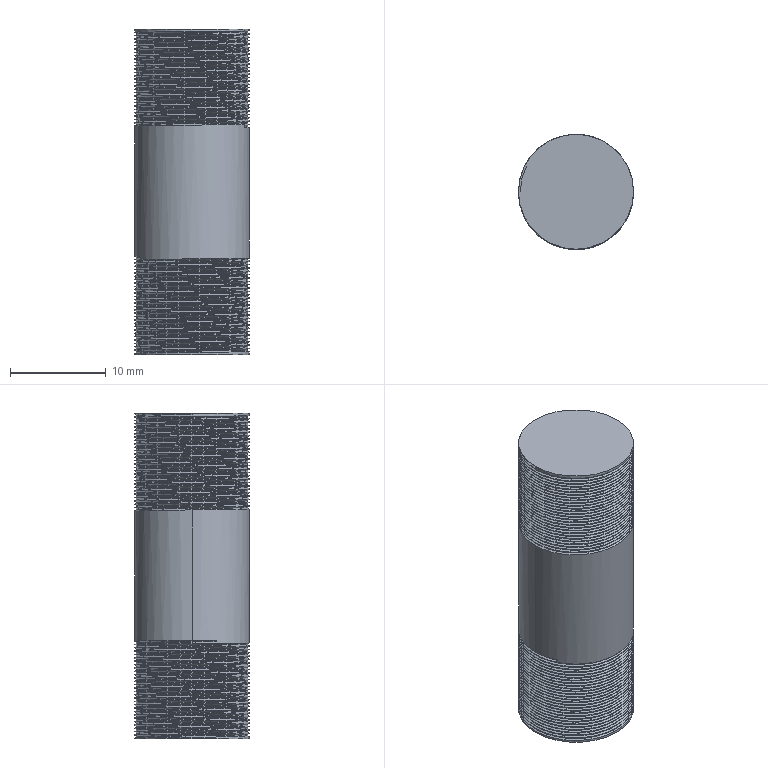Part | STEP file | Hinge seat cylinder 1 | 1 solid | 128 faces | box 12 x 12 x 34 mm | volume 3769 mm3 | cylinder 116 | plane 6 | spline 6 | commonest cylinder face diameters 12 x116